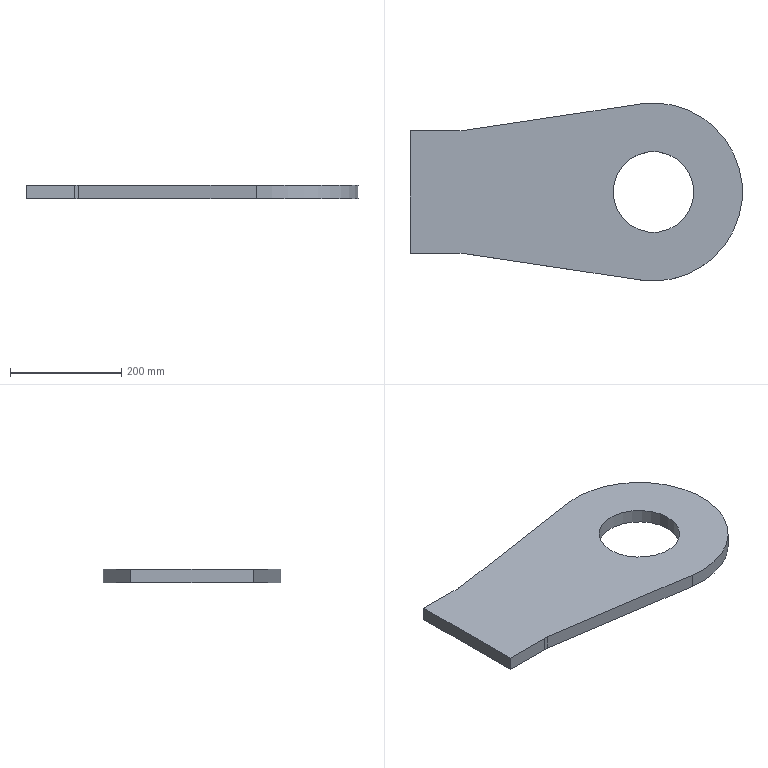Part | NX | features 前连杆 2 | 1 solid | 11 faces | box 597.539 x 319.958 x 25 mm | volume 3444700 mm3 | plane 7 | cylinder 4 | commonest cylinder face diameters 200 x2 145 x1 319.958 x1
STEP:
#1=CARTESIAN_POINT('',(1490.797,-110.28,320.));
#2=VERTEX_POINT('',#1);
#3=CARTESIAN_POINT('',(1483.315,-110.,320.));
#4=VERTEX_POINT('',#3);
#5=CARTESIAN_POINT('',(1483.315,-210.,320.));
#6=DIRECTION('',(0.,0.,1.));
#7=DIRECTION('',(1.,0.,0.));
#8=AXIS2_PLACEMENT_3D('',#5,#6,#7);
#9=CIRCLE('',#8,100.);
#10=EDGE_CURVE('',#2,#4,#9,.T.);
#11=ORIENTED_EDGE('',*,*,#10,.T.);
#12=CARTESIAN_POINT('',(1483.315,-110.,295.));
#13=VERTEX_POINT('',#12);
#14=CARTESIAN_POINT('',(1483.315,-110.,295.));
#15=DIRECTION('',(0.,0.,1.));
#16=VECTOR('',#15,1000.);
#17=LINE('',#14,#16);
#18=EDGE_CURVE('',#13,#4,#17,.T.);
#19=ORIENTED_EDGE('',*,*,#18,.F.);
#20=CARTESIAN_POINT('',(1490.797,-110.28,295.));
#21=VERTEX_POINT('',#20);
#22=CARTESIAN_POINT('',(1483.315,-210.,295.));
#23=DIRECTION('',(0.,0.,1.));
#24=DIRECTION('',(1.,0.,0.));
#25=AXIS2_PLACEMENT_3D('',#22,#23,#24);
#26=CIRCLE('',#25,100.);
#27=EDGE_CURVE('',#21,#13,#26,.T.);
#28=ORIENTED_EDGE('',*,*,#27,.F.);
#29=CARTESIAN_POINT('',(1490.797,-110.28,295.));
#30=DIRECTION('',(0.,0.,1.));
#31=VECTOR('',#30,1000.);
#32=LINE('',#29,#31);
#33=EDGE_CURVE('',#21,#2,#32,.T.);
#34=ORIENTED_EDGE('',*,*,#33,.T.);
#35=EDGE_LOOP('',(#11,#19,#28,#34));
#36=FACE_BOUND('',#35,.T.);
#37=CARTESIAN_POINT('',(1483.315,-210.,295.));
#38=DIRECTION('',(0.,0.,1.));
#39=DIRECTION('',(1.,0.,0.));
#40=AXIS2_PLACEMENT_3D('',#37,#38,#39);
#41=CYLINDRICAL_SURFACE('',#40,100.);
#42=ADVANCED_FACE('',(#36),#41,.F.);
#43=CARTESIAN_POINT('',(1396.428,-110.,320.));
#44=VERTEX_POINT('',#43);
#45=CARTESIAN_POINT('',(1483.315,-110.,320.));
#46=DIRECTION('',(-1.,0.,0.));
#47=VECTOR('',#46,1000.);
#48=LINE('',#45,#47);
#49=EDGE_CURVE('',#4,#44,#48,.T.);
#50=ORIENTED_EDGE('',*,*,#49,.T.);
#51=CARTESIAN_POINT('',(1396.428,-110.,295.));
#52=VERTEX_POINT('',#51);
#53=CARTESIAN_POINT('',(1396.428,-110.,295.));
#54=DIRECTION('',(0.,0.,1.));
#55=VECTOR('',#54,1000.);
#56=LINE('',#53,#55);
#57=EDGE_CURVE('',#52,#44,#56,.T.);
#58=ORIENTED_EDGE('',*,*,#57,.F.);
#59=CARTESIAN_POINT('',(1483.315,-110.,295.));
#60=DIRECTION('',(-1.,0.,0.));
#61=VECTOR('',#60,1000.);
#62=LINE('',#59,#61);
#63=EDGE_CURVE('',#13,#52,#62,.T.);
#64=ORIENTED_EDGE('',*,*,#63,.F.);
#65=ORIENTED_EDGE('',*,*,#18,.T.);
#66=EDGE_LOOP('',(#50,#58,#64,#65));
#67=FACE_BOUND('',#66,.T.);
#68=CARTESIAN_POINT('',(1483.315,-110.,295.));
#69=DIRECTION('',(0.,1.,0.));
#70=DIRECTION('',(0.,0.,1.));
#71=AXIS2_PLACEMENT_3D('',#68,#69,#70);
#72=PLANE('',#71);
#73=ADVANCED_FACE('',(#67),#72,.F.);
#74=CARTESIAN_POINT('',(1396.428,110.,320.));
#75=VERTEX_POINT('',#74);
#76=CARTESIAN_POINT('',(1396.428,-110.,320.));
#77=DIRECTION('',(0.,1.,0.));
#78=VECTOR('',#77,1000.);
#79=LINE('',#76,#78);
#80=EDGE_CURVE('',#44,#75,#79,.T.);
#81=ORIENTED_EDGE('',*,*,#80,.T.);
#82=CARTESIAN_POINT('',(1396.428,110.,295.));
#83=VERTEX_POINT('',#82);
#84=CARTESIAN_POINT('',(1396.428,110.,295.));
#85=DIRECTION('',(0.,0.,1.));
#86=VECTOR('',#85,1000.);
#87=LINE('',#84,#86);
#88=EDGE_CURVE('',#83,#75,#87,.T.);
#89=ORIENTED_EDGE('',*,*,#88,.F.);
#90=CARTESIAN_POINT('',(1396.428,-110.,295.));
#91=DIRECTION('',(0.,1.,0.));
#92=VECTOR('',#91,1000.);
#93=LINE('',#90,#92);
#94=EDGE_CURVE('',#52,#83,#93,.T.);
#95=ORIENTED_EDGE('',*,*,#94,.F.);
#96=ORIENTED_EDGE('',*,*,#57,.T.);
#97=EDGE_LOOP('',(#81,#89,#95,#96));
#98=FACE_BOUND('',#97,.T.);
#99=CARTESIAN_POINT('',(1396.428,-110.,295.));
#100=DIRECTION('',(1.,0.,0.));
#101=DIRECTION('',(0.,0.,-1.));
#102=AXIS2_PLACEMENT_3D('',#99,#100,#101);
#103=PLANE('',#102);
#104=ADVANCED_FACE('',(#98),#103,.F.);
#105=CARTESIAN_POINT('',(1483.315,110.,320.));
#106=VERTEX_POINT('',#105);
#107=CARTESIAN_POINT('',(1396.428,110.,320.));
#108=DIRECTION('',(1.,0.,0.));
#109=VECTOR('',#108,1000.);
#110=LINE('',#107,#109);
#111=EDGE_CURVE('',#75,#106,#110,.T.);
#112=ORIENTED_EDGE('',*,*,#111,.T.);
#113=CARTESIAN_POINT('',(1483.315,110.,295.));
#114=VERTEX_POINT('',#113);
#115=CARTESIAN_POINT('',(1483.315,110.,295.));
#116=DIRECTION('',(0.,0.,1.));
#117=VECTOR('',#116,1000.);
#118=LINE('',#115,#117);
#119=EDGE_CURVE('',#114,#106,#118,.T.);
#120=ORIENTED_EDGE('',*,*,#119,.F.);
#121=CARTESIAN_POINT('',(1396.428,110.,295.));
#122=DIRECTION('',(1.,0.,0.));
#123=VECTOR('',#122,1000.);
#124=LINE('',#121,#123);
#125=EDGE_CURVE('',#83,#114,#124,.T.);
#126=ORIENTED_EDGE('',*,*,#125,.F.);
#127=ORIENTED_EDGE('',*,*,#88,.T.);
#128=EDGE_LOOP('',(#112,#120,#126,#127));
#129=FACE_BOUND('',#128,.T.);
#130=CARTESIAN_POINT('',(1396.428,110.,295.));
#131=DIRECTION('',(0.,-1.,0.));
#132=DIRECTION('',(0.,0.,-1.));
#133=AXIS2_PLACEMENT_3D('',#130,#131,#132);
#134=PLANE('',#133);
#135=ADVANCED_FACE('',(#129),#134,.F.);
#136=CARTESIAN_POINT('',(1490.797,110.28,320.));
#137=VERTEX_POINT('',#136);
#138=CARTESIAN_POINT('',(1483.315,210.,320.));
#139=DIRECTION('',(0.,0.,1.));
#140=DIRECTION('',(1.,0.,0.));
#141=AXIS2_PLACEMENT_3D('',#138,#139,#140);
#142=CIRCLE('',#141,100.);
#143=EDGE_CURVE('',#106,#137,#142,.T.);
#144=ORIENTED_EDGE('',*,*,#143,.T.);
#145=CARTESIAN_POINT('',(1490.797,110.28,295.));
#146=VERTEX_POINT('',#145);
#147=CARTESIAN_POINT('',(1490.797,110.28,295.));
#148=DIRECTION('',(0.,0.,1.));
#149=VECTOR('',#148,1000.);
#150=LINE('',#147,#149);
#151=EDGE_CURVE('',#146,#137,#150,.T.);
#152=ORIENTED_EDGE('',*,*,#151,.F.);
#153=CARTESIAN_POINT('',(1483.315,210.,295.));
#154=DIRECTION('',(0.,0.,1.));
#155=DIRECTION('',(1.,0.,0.));
#156=AXIS2_PLACEMENT_3D('',#153,#154,#155);
#157=CIRCLE('',#156,100.);
#158=EDGE_CURVE('',#114,#146,#157,.T.);
#159=ORIENTED_EDGE('',*,*,#158,.F.);
#160=ORIENTED_EDGE('',*,*,#119,.T.);
#161=EDGE_LOOP('',(#144,#152,#159,#160));
#162=FACE_BOUND('',#161,.T.);
#163=CARTESIAN_POINT('',(1483.315,210.,295.));
#164=DIRECTION('',(0.,0.,1.));
#165=DIRECTION('',(1.,0.,0.));
#166=AXIS2_PLACEMENT_3D('',#163,#164,#165);
#167=CYLINDRICAL_SURFACE('',#166,100.);
#168=ADVANCED_FACE('',(#162),#167,.F.);
#169=CARTESIAN_POINT('',(1810.252,158.208,320.));
#170=VERTEX_POINT('',#169);
#171=CARTESIAN_POINT('',(1490.797,110.28,320.));
#172=DIRECTION('',(0.9889,0.1484,0.));
#173=VECTOR('',#172,1000.);
#174=LINE('',#171,#173);
#175=EDGE_CURVE('',#137,#170,#174,.T.);
#176=ORIENTED_EDGE('',*,*,#175,.T.);
#177=CARTESIAN_POINT('',(1810.252,158.208,295.));
#178=VERTEX_POINT('',#177);
#179=CARTESIAN_POINT('',(1810.252,158.208,295.));
#180=DIRECTION('',(0.,0.,1.));
#181=VECTOR('',#180,1000.);
#182=LINE('',#179,#181);
#183=EDGE_CURVE('',#178,#170,#182,.T.);
#184=ORIENTED_EDGE('',*,*,#183,.F.);
#185=CARTESIAN_POINT('',(1490.797,110.28,295.));
#186=DIRECTION('',(0.9889,0.1484,0.));
#187=VECTOR('',#186,1000.);
#188=LINE('',#185,#187);
#189=EDGE_CURVE('',#146,#178,#188,.T.);
#190=ORIENTED_EDGE('',*,*,#189,.F.);
#191=ORIENTED_EDGE('',*,*,#151,.T.);
#192=EDGE_LOOP('',(#176,#184,#190,#191));
#193=FACE_BOUND('',#192,.T.);
#194=CARTESIAN_POINT('',(1490.797,110.28,295.));
#195=DIRECTION('',(0.1484,-0.9889,0.));
#196=DIRECTION('',(0.9889,0.1484,0.));
#197=AXIS2_PLACEMENT_3D('',#194,#195,#196);
#198=PLANE('',#197);
#199=ADVANCED_FACE('',(#193),#198,.F.);
#200=CARTESIAN_POINT('',(1810.252,-158.208,320.));
#201=VERTEX_POINT('',#200);
#202=CARTESIAN_POINT('',(1833.988,0.,320.));
#203=DIRECTION('',(0.,0.,-1.));
#204=DIRECTION('',(-1.,0.,0.));
#205=AXIS2_PLACEMENT_3D('',#202,#203,#204);
#206=CIRCLE('',#205,159.979);
#207=EDGE_CURVE('',#170,#201,#206,.T.);
#208=ORIENTED_EDGE('',*,*,#207,.T.);
#209=CARTESIAN_POINT('',(1810.252,-158.208,295.));
#210=VERTEX_POINT('',#209);
#211=CARTESIAN_POINT('',(1810.252,-158.208,295.));
#212=DIRECTION('',(0.,0.,1.));
#213=VECTOR('',#212,1000.);
#214=LINE('',#211,#213);
#215=EDGE_CURVE('',#210,#201,#214,.T.);
#216=ORIENTED_EDGE('',*,*,#215,.F.);
#217=CARTESIAN_POINT('',(1833.988,0.,295.));
#218=DIRECTION('',(0.,0.,-1.));
#219=DIRECTION('',(-1.,0.,0.));
#220=AXIS2_PLACEMENT_3D('',#217,#218,#219);
#221=CIRCLE('',#220,159.979);
#222=EDGE_CURVE('',#178,#210,#221,.T.);
#223=ORIENTED_EDGE('',*,*,#222,.F.);
#224=ORIENTED_EDGE('',*,*,#183,.T.);
#225=EDGE_LOOP('',(#208,#216,#223,#224));
#226=FACE_BOUND('',#225,.T.);
#227=CARTESIAN_POINT('',(1833.988,0.,295.));
#228=DIRECTION('',(0.,0.,1.));
#229=DIRECTION('',(1.,0.,0.));
#230=AXIS2_PLACEMENT_3D('',#227,#228,#229);
#231=CYLINDRICAL_SURFACE('',#230,159.979);
#232=ADVANCED_FACE('',(#226),#231,.T.);
#233=CARTESIAN_POINT('',(1810.252,-158.208,320.));
#234=DIRECTION('',(-0.9889,0.1484,0.));
#235=VECTOR('',#234,1000.);
#236=LINE('',#233,#235);
#237=EDGE_CURVE('',#201,#2,#236,.T.);
#238=ORIENTED_EDGE('',*,*,#237,.T.);
#239=ORIENTED_EDGE('',*,*,#33,.F.);
#240=CARTESIAN_POINT('',(1810.252,-158.208,295.));
#241=DIRECTION('',(-0.9889,0.1484,0.));
#242=VECTOR('',#241,1000.);
#243=LINE('',#240,#242);
#244=EDGE_CURVE('',#210,#21,#243,.T.);
#245=ORIENTED_EDGE('',*,*,#244,.F.);
#246=ORIENTED_EDGE('',*,*,#215,.T.);
#247=EDGE_LOOP('',(#238,#239,#245,#246));
#248=FACE_BOUND('',#247,.T.);
#249=CARTESIAN_POINT('',(1810.252,-158.208,295.));
#250=DIRECTION('',(0.1484,0.9889,0.));
#251=DIRECTION('',(-0.9889,0.1484,0.));
#252=AXIS2_PLACEMENT_3D('',#249,#250,#251);
#253=PLANE('',#252);
#254=ADVANCED_FACE('',(#248),#253,.F.);
#255=CARTESIAN_POINT('',(1906.628,0.,295.));
#256=VERTEX_POINT('',#255);
#257=CARTESIAN_POINT('',(1834.128,0.,295.));
#258=DIRECTION('',(0.,0.,1.));
#259=DIRECTION('',(1.,0.,0.));
#260=AXIS2_PLACEMENT_3D('',#257,#258,#259);
#261=CIRCLE('',#260,72.5);
#262=EDGE_CURVE('',#256,#256,#261,.T.);
#263=ORIENTED_EDGE('',*,*,#262,.T.);
#264=EDGE_LOOP('',(#263));
#265=FACE_BOUND('',#264,.T.);
#266=ORIENTED_EDGE('',*,*,#27,.T.);
#267=ORIENTED_EDGE('',*,*,#63,.T.);
#268=ORIENTED_EDGE('',*,*,#94,.T.);
#269=ORIENTED_EDGE('',*,*,#125,.T.);
#270=ORIENTED_EDGE('',*,*,#158,.T.);
#271=ORIENTED_EDGE('',*,*,#189,.T.);
#272=ORIENTED_EDGE('',*,*,#222,.T.);
#273=ORIENTED_EDGE('',*,*,#244,.T.);
#274=EDGE_LOOP('',(#266,#267,#268,#269,#270,#271,#272,#273));
#275=FACE_BOUND('',#274,.T.);
#276=CARTESIAN_POINT('',(1483.315,-210.,295.));
#277=DIRECTION('',(0.,0.,1.));
#278=DIRECTION('',(1.,0.,0.));
#279=AXIS2_PLACEMENT_3D('',#276,#277,#278);
#280=PLANE('',#279);
#281=ADVANCED_FACE('',(#265,#275),#280,.F.);
#282=CARTESIAN_POINT('',(1906.628,0.,320.));
#283=VERTEX_POINT('',#282);
#284=CARTESIAN_POINT('',(1834.128,0.,320.));
#285=DIRECTION('',(0.,0.,1.));
#286=DIRECTION('',(1.,0.,0.));
#287=AXIS2_PLACEMENT_3D('',#284,#285,#286);
#288=CIRCLE('',#287,72.5);
#289=EDGE_CURVE('',#283,#283,#288,.T.);
#290=ORIENTED_EDGE('',*,*,#289,.F.);
#291=EDGE_LOOP('',(#290));
#292=FACE_BOUND('',#291,.T.);
#293=ORIENTED_EDGE('',*,*,#10,.F.);
#294=ORIENTED_EDGE('',*,*,#237,.F.);
#295=ORIENTED_EDGE('',*,*,#207,.F.);
#296=ORIENTED_EDGE('',*,*,#175,.F.);
#297=ORIENTED_EDGE('',*,*,#143,.F.);
#298=ORIENTED_EDGE('',*,*,#111,.F.);
#299=ORIENTED_EDGE('',*,*,#80,.F.);
#300=ORIENTED_EDGE('',*,*,#49,.F.);
#301=EDGE_LOOP('',(#293,#294,#295,#296,#297,#298,#299,#300));
#302=FACE_BOUND('',#301,.T.);
#303=CARTESIAN_POINT('',(1483.315,-210.,320.));
#304=DIRECTION('',(0.,0.,1.));
#305=DIRECTION('',(1.,0.,0.));
#306=AXIS2_PLACEMENT_3D('',#303,#304,#305);
#307=PLANE('',#306);
#308=ADVANCED_FACE('',(#292,#302),#307,.T.);
#309=ORIENTED_EDGE('',*,*,#289,.T.);
#310=EDGE_LOOP('',(#309));
#311=FACE_BOUND('',#310,.T.);
#312=ORIENTED_EDGE('',*,*,#262,.F.);
#313=EDGE_LOOP('',(#312));
#314=FACE_BOUND('',#313,.T.);
#315=CARTESIAN_POINT('',(1834.128,0.,345.));
#316=DIRECTION('',(0.,0.,-1.));
#317=DIRECTION('',(-1.,0.,0.));
#318=AXIS2_PLACEMENT_3D('',#315,#316,#317);
#319=CYLINDRICAL_SURFACE('',#318,72.5);
#320=ADVANCED_FACE('',(#311,#314),#319,.F.);
#321=CLOSED_SHELL('',(#42,#73,#104,#135,#168,#199,#232,#254,#281,#308,#320));
#322=MANIFOLD_SOLID_BREP('',#321);
#323=(LENGTH_UNIT()NAMED_UNIT(*)SI_UNIT(.MILLI.,.METRE.));
#324=UNCERTAINTY_MEASURE_WITH_UNIT(LENGTH_MEASURE(0.00001),#323,'','');
#325=(NAMED_UNIT(*)PLANE_ANGLE_UNIT()SI_UNIT($,.RADIAN.));
#326=(NAMED_UNIT(*)SI_UNIT($,.STERADIAN.)SOLID_ANGLE_UNIT());
#327=(GEOMETRIC_REPRESENTATION_CONTEXT(3)GLOBAL_UNCERTAINTY_ASSIGNED_CONTEXT((#324))GLOBAL_UNIT_ASSIGNED_CONTEXT((#323,#325,#326))REPRESENTATION_CONTEXT('',''));
#328=ADVANCED_BREP_SHAPE_REPRESENTATION('',(#322),#327);